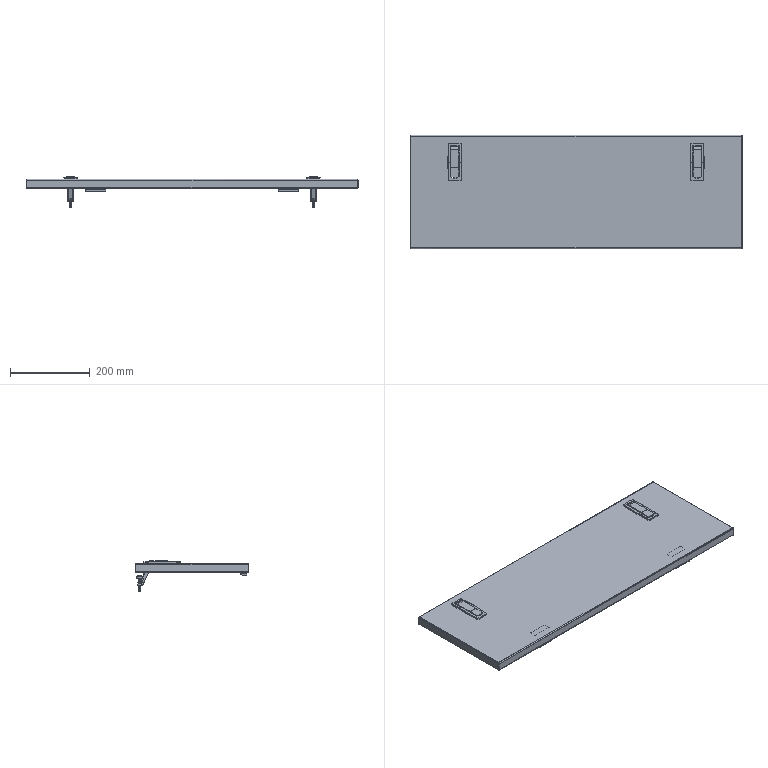Part | SolidWorks | features ReferencePattern 2, MirrorCompFeat 1 | 9 solids | 1112 faces | box 834 x 286 x 75.7 mm | volume 533972 mm3 | cylinder 522 | plane 330 | spline 186 | torus 62 | sphere 8 | cone 4 | commonest cylinder face diameters 4.8 x240 0.4 x60 3.2 x28 0.692 x24 4 x20 12.8 x20